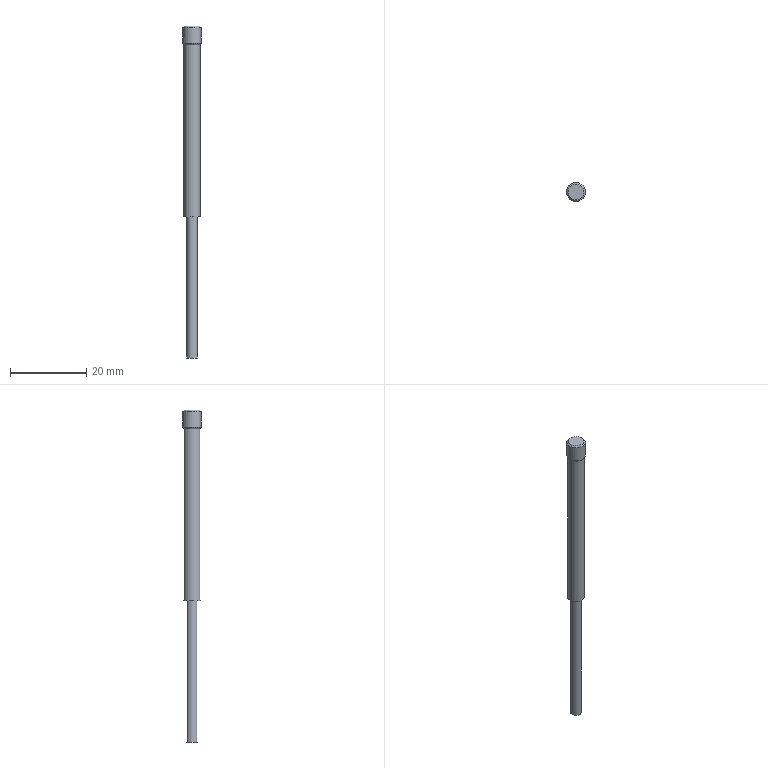Part | NX | features MI_APJAL_0242 2 | 1 solid | 9 faces | box 4.9 x 4.9 x 87 mm | volume 1004 mm3 | cylinder 3 | plane 3 | spline 2 | cone 1 | commonest cylinder face diameters 2.8 x1 4.4 x1 4.9 x1
STEP:
#1=CARTESIAN_POINT('',(146.8,-140.,73.1));
#2=VERTEX_POINT('',#1);
#3=CARTESIAN_POINT('',(151.2,-140.,73.1));
#4=VERTEX_POINT('',#3);
#5=CARTESIAN_POINT('',(149.,-140.,73.1));
#6=DIRECTION('',(0.,0.,1.));
#7=DIRECTION('',(1.,0.,0.));
#8=AXIS2_PLACEMENT_3D('',#5,#6,#7);
#9=CIRCLE('',#8,2.2);
#10=EDGE_CURVE('',#2,#4,#9,.T.);
#11=ORIENTED_EDGE('',*,*,#10,.T.);
#12=CARTESIAN_POINT('',(151.2,-139.998,73.1));
#13=VERTEX_POINT('',#12);
#14=CARTESIAN_POINT('',(149.,-140.,73.1));
#15=DIRECTION('',(0.,0.,1.));
#16=DIRECTION('',(1.,0.,0.));
#17=AXIS2_PLACEMENT_3D('',#14,#15,#16);
#18=CIRCLE('',#17,2.2);
#19=EDGE_CURVE('',#4,#13,#18,.T.);
#20=ORIENTED_EDGE('',*,*,#19,.T.);
#21=CARTESIAN_POINT('',(151.45,-139.998,73.448));
#22=VERTEX_POINT('',#21);
#23=CARTESIAN_POINT('',(151.45,-139.998,73.448));
#24=DIRECTION('',(-0.5832,-0.0004724,-0.8123));
#25=VECTOR('',#24,1000.);
#26=LINE('',#23,#25);
#27=EDGE_CURVE('',#22,#13,#26,.T.);
#28=ORIENTED_EDGE('',*,*,#27,.F.);
#29=CARTESIAN_POINT('',(151.45,-140.,73.448));
#30=VERTEX_POINT('',#29);
#31=CARTESIAN_POINT('',(151.45,-139.998,73.448));
#32=CARTESIAN_POINT('',(151.45,-139.999,73.448));
#33=CARTESIAN_POINT('',(151.45,-139.999,73.448));
#34=CARTESIAN_POINT('',(151.45,-140.,73.448));
#35=B_SPLINE_CURVE_WITH_KNOTS('',3,(#31,#32,#33,#34),.UNSPECIFIED.,.F.,.F.,(4,4),(13.004,13.006),.UNSPECIFIED.);
#36=EDGE_CURVE('',#22,#30,#35,.T.);
#37=ORIENTED_EDGE('',*,*,#36,.T.);
#38=CARTESIAN_POINT('',(148.979,-142.45,73.448));
#39=VERTEX_POINT('',#38);
#40=CARTESIAN_POINT('',(151.45,-140.,73.448));
#41=CARTESIAN_POINT('',(151.45,-140.316,73.448));
#42=CARTESIAN_POINT('',(151.387,-140.638,73.448));
#43=CARTESIAN_POINT('',(151.147,-141.223,73.448));
#44=CARTESIAN_POINT('',(150.966,-141.496,73.448));
#45=CARTESIAN_POINT('',(150.522,-141.946,73.448));
#46=CARTESIAN_POINT('',(150.251,-142.13,73.448));
#47=CARTESIAN_POINT('',(149.669,-142.378,73.448));
#48=CARTESIAN_POINT('',(149.348,-142.446,73.448));
#49=CARTESIAN_POINT('',(149.014,-142.45,73.448));
#50=CARTESIAN_POINT('',(148.996,-142.45,73.448));
#51=CARTESIAN_POINT('',(148.979,-142.45,73.448));
#52=B_SPLINE_CURVE_WITH_KNOTS('',3,(#40,#41,#42,#43,#44,#45,#46,#47,#48,#49,#50,#51),.UNSPECIFIED.,.F.,.F.,(4,2,2,2,2,4),(0.,0.8058,1.612,2.418,3.223,3.269),.UNSPECIFIED.);
#53=EDGE_CURVE('',#30,#39,#52,.T.);
#54=ORIENTED_EDGE('',*,*,#53,.T.);
#55=CARTESIAN_POINT('',(146.55,-140.,73.448));
#56=VERTEX_POINT('',#55);
#57=CARTESIAN_POINT('',(148.979,-142.45,73.448));
#58=CARTESIAN_POINT('',(148.68,-142.447,73.448));
#59=CARTESIAN_POINT('',(148.377,-142.388,73.448));
#60=CARTESIAN_POINT('',(147.806,-142.162,73.448));
#61=CARTESIAN_POINT('',(147.53,-141.985,73.448));
#62=CARTESIAN_POINT('',(147.074,-141.547,73.448));
#63=CARTESIAN_POINT('',(146.886,-141.278,73.448));
#64=CARTESIAN_POINT('',(146.631,-140.7,73.448));
#65=CARTESIAN_POINT('',(146.559,-140.38,73.448));
#66=CARTESIAN_POINT('',(146.55,-140.043,73.448));
#67=CARTESIAN_POINT('',(146.55,-140.021,73.448));
#68=CARTESIAN_POINT('',(146.55,-140.,73.448));
#69=B_SPLINE_CURVE_WITH_KNOTS('',3,(#57,#58,#59,#60,#61,#62,#63,#64,#65,#66,#67,#68),.UNSPECIFIED.,.F.,.F.,(4,2,2,2,2,4),(3.269,4.029,4.835,5.641,6.447,6.501),.UNSPECIFIED.);
#70=EDGE_CURVE('',#39,#56,#69,.T.);
#71=ORIENTED_EDGE('',*,*,#70,.T.);
#72=CARTESIAN_POINT('',(146.8,-140.,73.1));
#73=CARTESIAN_POINT('',(146.717,-140.,73.216));
#74=CARTESIAN_POINT('',(146.634,-140.,73.332));
#75=CARTESIAN_POINT('',(146.55,-140.,73.449));
#76=B_SPLINE_CURVE_WITH_KNOTS('',3,(#72,#73,#74,#75),.UNSPECIFIED.,.F.,.F.,(4,4),(0.,1.),.UNSPECIFIED.);
#77=EDGE_CURVE('',#2,#56,#76,.T.);
#78=ORIENTED_EDGE('',*,*,#77,.F.);
#79=EDGE_LOOP('',(#11,#20,#28,#37,#54,#71,#78));
#80=FACE_BOUND('',#79,.T.);
#81=CARTESIAN_POINT('',(146.8,-140.,73.1));
#82=CARTESIAN_POINT('',(146.717,-140.,73.216));
#83=CARTESIAN_POINT('',(146.634,-140.,73.332));
#84=CARTESIAN_POINT('',(146.55,-140.,73.449));
#85=CARTESIAN_POINT('',(146.8,-140.162,73.1));
#86=CARTESIAN_POINT('',(146.717,-140.168,73.216));
#87=CARTESIAN_POINT('',(146.634,-140.174,73.332));
#88=CARTESIAN_POINT('',(146.55,-140.18,73.449));
#89=CARTESIAN_POINT('',(146.818,-140.324,73.1));
#90=CARTESIAN_POINT('',(146.736,-140.337,73.216));
#91=CARTESIAN_POINT('',(146.653,-140.349,73.332));
#92=CARTESIAN_POINT('',(146.571,-140.361,73.449));
#93=CARTESIAN_POINT('',(146.889,-140.64,73.1));
#94=CARTESIAN_POINT('',(146.809,-140.664,73.216));
#95=CARTESIAN_POINT('',(146.729,-140.688,73.332));
#96=CARTESIAN_POINT('',(146.65,-140.713,73.449));
#97=CARTESIAN_POINT('',(146.943,-140.795,73.1));
#98=CARTESIAN_POINT('',(146.865,-140.825,73.216));
#99=CARTESIAN_POINT('',(146.787,-140.855,73.332));
#100=CARTESIAN_POINT('',(146.709,-140.885,73.449));
#101=CARTESIAN_POINT('',(147.133,-141.197,73.1));
#102=CARTESIAN_POINT('',(147.062,-141.243,73.216));
#103=CARTESIAN_POINT('',(146.992,-141.288,73.332));
#104=CARTESIAN_POINT('',(146.921,-141.333,73.449));
#105=CARTESIAN_POINT('',(147.308,-141.434,73.1));
#106=CARTESIAN_POINT('',(147.244,-141.489,73.216));
#107=CARTESIAN_POINT('',(147.18,-141.543,73.332));
#108=CARTESIAN_POINT('',(147.116,-141.597,73.449));
#109=CARTESIAN_POINT('',(147.728,-141.817,73.1));
#110=CARTESIAN_POINT('',(147.679,-141.885,73.216));
#111=CARTESIAN_POINT('',(147.631,-141.954,73.332));
#112=CARTESIAN_POINT('',(147.583,-142.023,73.448));
#113=CARTESIAN_POINT('',(147.98,-141.969,73.1));
#114=CARTESIAN_POINT('',(147.941,-142.044,73.216));
#115=CARTESIAN_POINT('',(147.902,-142.118,73.332));
#116=CARTESIAN_POINT('',(147.864,-142.193,73.448));
#117=CARTESIAN_POINT('',(148.513,-142.164,73.1));
#118=CARTESIAN_POINT('',(148.494,-142.246,73.216));
#119=CARTESIAN_POINT('',(148.476,-142.328,73.332));
#120=CARTESIAN_POINT('',(148.457,-142.41,73.448));
#121=CARTESIAN_POINT('',(148.804,-142.209,73.1));
#122=CARTESIAN_POINT('',(148.796,-142.293,73.216));
#123=CARTESIAN_POINT('',(148.789,-142.377,73.332));
#124=CARTESIAN_POINT('',(148.781,-142.46,73.448));
#125=CARTESIAN_POINT('',(149.371,-142.187,73.1));
#126=CARTESIAN_POINT('',(149.385,-142.27,73.216));
#127=CARTESIAN_POINT('',(149.399,-142.353,73.332));
#128=CARTESIAN_POINT('',(149.413,-142.435,73.448));
#129=CARTESIAN_POINT('',(149.657,-142.119,73.1));
#130=CARTESIAN_POINT('',(149.682,-142.199,73.216));
#131=CARTESIAN_POINT('',(149.707,-142.279,73.332));
#132=CARTESIAN_POINT('',(149.732,-142.359,73.448));
#133=CARTESIAN_POINT('',(150.173,-141.883,73.1));
#134=CARTESIAN_POINT('',(150.218,-141.954,73.216));
#135=CARTESIAN_POINT('',(150.262,-142.025,73.332));
#136=CARTESIAN_POINT('',(150.307,-142.097,73.448));
#137=CARTESIAN_POINT('',(150.412,-141.711,73.1));
#138=CARTESIAN_POINT('',(150.466,-141.775,73.216));
#139=CARTESIAN_POINT('',(150.519,-141.84,73.332));
#140=CARTESIAN_POINT('',(150.573,-141.905,73.448));
#141=CARTESIAN_POINT('',(150.8,-141.296,73.1));
#142=CARTESIAN_POINT('',(150.868,-141.345,73.216));
#143=CARTESIAN_POINT('',(150.937,-141.395,73.332));
#144=CARTESIAN_POINT('',(151.005,-141.444,73.448));
#145=CARTESIAN_POINT('',(150.956,-141.046,73.1));
#146=CARTESIAN_POINT('',(151.03,-141.086,73.216));
#147=CARTESIAN_POINT('',(151.104,-141.126,73.332));
#148=CARTESIAN_POINT('',(151.178,-141.165,73.448));
#149=CARTESIAN_POINT('',(151.158,-140.516,73.1));
#150=CARTESIAN_POINT('',(151.239,-140.535,73.216));
#151=CARTESIAN_POINT('',(151.321,-140.555,73.332));
#152=CARTESIAN_POINT('',(151.403,-140.575,73.448));
#153=CARTESIAN_POINT('',(151.207,-140.226,73.1));
#154=CARTESIAN_POINT('',(151.291,-140.234,73.216));
#155=CARTESIAN_POINT('',(151.374,-140.243,73.332));
#156=CARTESIAN_POINT('',(151.458,-140.251,73.448));
#157=CARTESIAN_POINT('',(151.192,-139.658,73.1));
#158=CARTESIAN_POINT('',(151.275,-139.645,73.216));
#159=CARTESIAN_POINT('',(151.358,-139.632,73.332));
#160=CARTESIAN_POINT('',(151.441,-139.619,73.448));
#161=CARTESIAN_POINT('',(151.128,-139.371,73.1));
#162=CARTESIAN_POINT('',(151.208,-139.347,73.216));
#163=CARTESIAN_POINT('',(151.289,-139.323,73.332));
#164=CARTESIAN_POINT('',(151.369,-139.299,73.448));
#165=CARTESIAN_POINT('',(150.898,-138.852,73.1));
#166=CARTESIAN_POINT('',(150.97,-138.808,73.216));
#167=CARTESIAN_POINT('',(151.042,-138.765,73.332));
#168=CARTESIAN_POINT('',(151.114,-138.721,73.448));
#169=CARTESIAN_POINT('',(150.73,-138.61,73.1));
#170=CARTESIAN_POINT('',(150.795,-138.558,73.216));
#171=CARTESIAN_POINT('',(150.861,-138.505,73.332));
#172=CARTESIAN_POINT('',(150.926,-138.452,73.448));
#173=CARTESIAN_POINT('',(150.32,-138.217,73.1));
#174=CARTESIAN_POINT('',(150.37,-138.15,73.216));
#175=CARTESIAN_POINT('',(150.42,-138.082,73.332));
#176=CARTESIAN_POINT('',(150.47,-138.014,73.448));
#177=CARTESIAN_POINT('',(150.073,-138.058,73.1));
#178=CARTESIAN_POINT('',(150.113,-137.984,73.216));
#179=CARTESIAN_POINT('',(150.154,-137.911,73.332));
#180=CARTESIAN_POINT('',(150.194,-137.837,73.448));
#181=CARTESIAN_POINT('',(149.545,-137.849,73.1));
#182=CARTESIAN_POINT('',(149.565,-137.768,73.216));
#183=CARTESIAN_POINT('',(149.586,-137.687,73.332));
#184=CARTESIAN_POINT('',(149.607,-137.605,73.448));
#185=CARTESIAN_POINT('',(149.255,-137.796,73.1));
#186=CARTESIAN_POINT('',(149.265,-137.713,73.216));
#187=CARTESIAN_POINT('',(149.274,-137.629,73.332));
#188=CARTESIAN_POINT('',(149.284,-137.546,73.448));
#189=CARTESIAN_POINT('',(148.688,-137.804,73.1));
#190=CARTESIAN_POINT('',(148.676,-137.721,73.216));
#191=CARTESIAN_POINT('',(148.664,-137.637,73.332));
#192=CARTESIAN_POINT('',(148.652,-137.554,73.448));
#193=CARTESIAN_POINT('',(148.399,-137.865,73.1));
#194=CARTESIAN_POINT('',(148.377,-137.784,73.216));
#195=CARTESIAN_POINT('',(148.354,-137.703,73.332));
#196=CARTESIAN_POINT('',(148.331,-137.622,73.448));
#197=CARTESIAN_POINT('',(147.877,-138.087,73.1));
#198=CARTESIAN_POINT('',(147.835,-138.015,73.216));
#199=CARTESIAN_POINT('',(147.792,-137.942,73.332));
#200=CARTESIAN_POINT('',(147.75,-137.87,73.448));
#201=CARTESIAN_POINT('',(147.634,-138.253,73.1));
#202=CARTESIAN_POINT('',(147.582,-138.186,73.216));
#203=CARTESIAN_POINT('',(147.53,-138.12,73.332));
#204=CARTESIAN_POINT('',(147.478,-138.054,73.448));
#205=CARTESIAN_POINT('',(147.235,-138.657,73.1));
#206=CARTESIAN_POINT('',(147.168,-138.606,73.216));
#207=CARTESIAN_POINT('',(147.101,-138.555,73.332));
#208=CARTESIAN_POINT('',(147.035,-138.504,73.448));
#209=CARTESIAN_POINT('',(147.073,-138.902,73.1));
#210=CARTESIAN_POINT('',(147.,-138.861,73.216));
#211=CARTESIAN_POINT('',(146.927,-138.819,73.332));
#212=CARTESIAN_POINT('',(146.854,-138.778,73.448));
#213=CARTESIAN_POINT('',(146.857,-139.427,73.1));
#214=CARTESIAN_POINT('',(146.776,-139.406,73.216));
#215=CARTESIAN_POINT('',(146.695,-139.384,73.332));
#216=CARTESIAN_POINT('',(146.614,-139.362,73.448));
#217=CARTESIAN_POINT('',(146.8,-139.716,73.1));
#218=CARTESIAN_POINT('',(146.717,-139.706,73.216));
#219=CARTESIAN_POINT('',(146.634,-139.695,73.332));
#220=CARTESIAN_POINT('',(146.55,-139.684,73.448));
#221=CARTESIAN_POINT('',(146.8,-140.,73.1));
#222=CARTESIAN_POINT('',(146.717,-140.,73.216));
#223=CARTESIAN_POINT('',(146.634,-140.,73.332));
#224=CARTESIAN_POINT('',(146.55,-140.,73.449));
#225=B_SPLINE_SURFACE_WITH_KNOTS('',3,3,((#81,#82,#83,#84),(#85,#86,#87,#88),(#89,#90,#91,#92),(#93,#94,#95,#96),(#97,#98,#99,#100),(#101,#102,#103,#104),(#105,#106,#107,#108),(#109,#110,#111,#112),(#113,#114,#115,#116),(#117,#118,#119,#120),(#121,#122,#123,#124),(#125,#126,#127,#128),(#129,#130,#131,#132),(#133,#134,#135,#136),(#137,#138,#139,#140),(#141,#142,#143,#144),(#145,#146,#147,#148),(#149,#150,#151,#152),(#153,#154,#155,#156),(#157,#158,#159,#160),(#161,#162,#163,#164),(#165,#166,#167,#168),(#169,#170,#171,#172),(#173,#174,#175,#176),(#177,#178,#179,#180),(#181,#182,#183,#184),(#185,#186,#187,#188),(#189,#190,#191,#192),(#193,#194,#195,#196),(#197,#198,#199,#200),(#201,#202,#203,#204),(#205,#206,#207,#208),(#209,#210,#211,#212),(#213,#214,#215,#216),(#217,#218,#219,#220),(#221,#222,#223,#224)),.RULED_SURF.,.T.,.F.,.F.,(4,2,2,2,2,2,2,2,2,2,2,2,2,2,2,2,2,4),(4,4),(-13.006,-12.547,-12.088,-11.282,-10.476,-9.67,-8.864,-8.058,-7.253,-6.447,-5.641,-4.835,-4.029,-3.223,-2.418,-1.612,-0.8058,0.),(0.,1.),.UNSPECIFIED.);
#226=ADVANCED_FACE('',(#80),#225,.T.);
#227=CARTESIAN_POINT('',(151.45,-140.014,77.632));
#228=VERTEX_POINT('',#227);
#229=CARTESIAN_POINT('',(146.55,-140.,77.632));
#230=VERTEX_POINT('',#229);
#231=CARTESIAN_POINT('',(149.,-140.,77.632));
#232=DIRECTION('',(0.,0.,1.));
#233=DIRECTION('',(-1.,0.,0.));
#234=AXIS2_PLACEMENT_3D('',#231,#232,#233);
#235=CIRCLE('',#234,2.45);
#236=EDGE_CURVE('',#228,#230,#235,.T.);
#237=ORIENTED_EDGE('',*,*,#236,.F.);
#238=CARTESIAN_POINT('',(148.979,-142.45,77.632));
#239=VERTEX_POINT('',#238);
#240=CARTESIAN_POINT('',(149.,-140.,77.632));
#241=DIRECTION('',(0.,0.,1.));
#242=DIRECTION('',(-1.,0.,0.));
#243=AXIS2_PLACEMENT_3D('',#240,#241,#242);
#244=CIRCLE('',#243,2.45);
#245=EDGE_CURVE('',#239,#228,#244,.T.);
#246=ORIENTED_EDGE('',*,*,#245,.F.);
#247=CARTESIAN_POINT('',(148.979,-142.45,77.632));
#248=CARTESIAN_POINT('',(148.979,-142.45,73.448));
#249=B_SPLINE_CURVE_WITH_KNOTS('',1,(#247,#248),.UNSPECIFIED.,.F.,.F.,(2,2),(0.08333,0.9167),.UNSPECIFIED.);
#250=EDGE_CURVE('',#239,#39,#249,.T.);
#251=ORIENTED_EDGE('',*,*,#250,.T.);
#252=ORIENTED_EDGE('',*,*,#53,.F.);
#253=ORIENTED_EDGE('',*,*,#36,.F.);
#254=CARTESIAN_POINT('',(146.55,-140.,73.448));
#255=CARTESIAN_POINT('',(146.55,-139.705,73.448));
#256=CARTESIAN_POINT('',(146.605,-139.405,73.448));
#257=CARTESIAN_POINT('',(146.822,-138.834,73.448));
#258=CARTESIAN_POINT('',(146.996,-138.556,73.448));
#259=CARTESIAN_POINT('',(147.428,-138.095,73.448));
#260=CARTESIAN_POINT('',(147.694,-137.903,73.448));
#261=CARTESIAN_POINT('',(148.269,-137.64,73.448));
#262=CARTESIAN_POINT('',(148.588,-137.564,73.448));
#263=CARTESIAN_POINT('',(149.219,-137.539,73.448));
#264=CARTESIAN_POINT('',(149.543,-137.59,73.448));
#265=CARTESIAN_POINT('',(150.137,-137.807,73.448));
#266=CARTESIAN_POINT('',(150.418,-137.977,73.448));
#267=CARTESIAN_POINT('',(150.885,-138.403,73.448));
#268=CARTESIAN_POINT('',(151.079,-138.667,73.448));
#269=CARTESIAN_POINT('',(151.292,-139.115,73.448));
#270=CARTESIAN_POINT('',(151.351,-139.287,73.448));
#271=CARTESIAN_POINT('',(151.43,-139.638,73.448));
#272=CARTESIAN_POINT('',(151.45,-139.819,73.448));
#273=CARTESIAN_POINT('',(151.45,-139.998,73.448));
#274=B_SPLINE_CURVE_WITH_KNOTS('',3,(#254,#255,#256,#257,#258,#259,#260,#261,#262,#263,#264,#265,#266,#267,#268,#269,#270,#271,#272,#273),.UNSPECIFIED.,.F.,.F.,(4,2,2,2,2,2,2,2,2,4),(6.501,7.253,8.058,8.864,9.67,10.476,11.282,12.088,12.547,13.004),.UNSPECIFIED.);
#275=EDGE_CURVE('',#56,#22,#274,.T.);
#276=ORIENTED_EDGE('',*,*,#275,.F.);
#277=ORIENTED_EDGE('',*,*,#70,.F.);
#278=ORIENTED_EDGE('',*,*,#250,.F.);
#279=CARTESIAN_POINT('',(149.,-140.,77.632));
#280=DIRECTION('',(0.,0.,1.));
#281=DIRECTION('',(-1.,0.,0.));
#282=AXIS2_PLACEMENT_3D('',#279,#280,#281);
#283=CIRCLE('',#282,2.45);
#284=EDGE_CURVE('',#230,#239,#283,.T.);
#285=ORIENTED_EDGE('',*,*,#284,.F.);
#286=EDGE_LOOP('',(#237,#246,#251,#252,#253,#276,#277,#278,#285));
#287=FACE_BOUND('',#286,.T.);
#288=CARTESIAN_POINT('',(149.,-140.,75.55));
#289=DIRECTION('',(0.,0.,-1.));
#290=DIRECTION('',(-0.008727,-1.,0.));
#291=AXIS2_PLACEMENT_3D('',#288,#289,#290);
#292=CYLINDRICAL_SURFACE('',#291,2.45);
#293=ADVANCED_FACE('',(#287),#292,.T.);
#294=CARTESIAN_POINT('',(146.917,-140.,78.));
#295=VERTEX_POINT('',#294);
#296=CARTESIAN_POINT('',(151.082,-140.012,78.));
#297=VERTEX_POINT('',#296);
#298=CARTESIAN_POINT('',(149.,-140.,78.));
#299=DIRECTION('',(0.,0.,-1.));
#300=DIRECTION('',(-1.,0.,0.));
#301=AXIS2_PLACEMENT_3D('',#298,#299,#300);
#302=CIRCLE('',#301,2.083);
#303=EDGE_CURVE('',#295,#297,#302,.T.);
#304=ORIENTED_EDGE('',*,*,#303,.T.);
#305=CARTESIAN_POINT('',(151.082,-140.012,78.));
#306=CARTESIAN_POINT('',(151.45,-140.014,77.633));
#307=B_SPLINE_CURVE_WITH_KNOTS('',1,(#305,#306),.UNSPECIFIED.,.F.,.F.,(2,2),(0.601,0.7071),.UNSPECIFIED.);
#308=EDGE_CURVE('',#297,#228,#307,.T.);
#309=ORIENTED_EDGE('',*,*,#308,.T.);
#310=ORIENTED_EDGE('',*,*,#236,.T.);
#311=ORIENTED_EDGE('',*,*,#284,.T.);
#312=ORIENTED_EDGE('',*,*,#245,.T.);
#313=ORIENTED_EDGE('',*,*,#308,.F.);
#314=CARTESIAN_POINT('',(149.,-140.,78.));
#315=DIRECTION('',(0.,0.,-1.));
#316=DIRECTION('',(-1.,0.,0.));
#317=AXIS2_PLACEMENT_3D('',#314,#315,#316);
#318=CIRCLE('',#317,2.083);
#319=EDGE_CURVE('',#297,#295,#318,.T.);
#320=ORIENTED_EDGE('',*,*,#319,.T.);
#321=EDGE_LOOP('',(#304,#309,#310,#311,#312,#313,#320));
#322=FACE_BOUND('',#321,.T.);
#323=CARTESIAN_POINT('',(149.,-140.,76.618));
#324=DIRECTION('',(0.,0.,-1.));
#325=DIRECTION('',(1.,-0.005818,0.));
#326=AXIS2_PLACEMENT_3D('',#323,#324,#325);
#327=CONICAL_SURFACE('',#326,3.465,0.7854);
#328=ADVANCED_FACE('',(#322),#327,.T.);
#329=ORIENTED_EDGE('',*,*,#319,.F.);
#330=ORIENTED_EDGE('',*,*,#303,.F.);
#331=EDGE_LOOP('',(#329,#330));
#332=FACE_BOUND('',#331,.T.);
#333=CARTESIAN_POINT('',(146.293,-144.328,78.));
#334=DIRECTION('',(0.,0.,1.));
#335=DIRECTION('',(1.,0.,0.));
#336=AXIS2_PLACEMENT_3D('',#333,#334,#335);
#337=PLANE('',#336);
#338=ADVANCED_FACE('',(#332),#337,.T.);
#339=CARTESIAN_POINT('',(147.6,-140.,28.));
#340=VERTEX_POINT('',#339);
#341=CARTESIAN_POINT('',(149.,-140.,28.));
#342=DIRECTION('',(0.,0.,1.));
#343=DIRECTION('',(-1.,0.,0.));
#344=AXIS2_PLACEMENT_3D('',#341,#342,#343);
#345=CIRCLE('',#344,1.4);
#346=EDGE_CURVE('',#340,#340,#345,.T.);
#347=ORIENTED_EDGE('',*,*,#346,.F.);
#348=CARTESIAN_POINT('',(147.6,-140.,-9.));
#349=VERTEX_POINT('',#348);
#350=CARTESIAN_POINT('',(147.6,-140.,28.));
#351=CARTESIAN_POINT('',(147.6,-140.,-9.));
#352=B_SPLINE_CURVE_WITH_KNOTS('',1,(#350,#351),.UNSPECIFIED.,.F.,.F.,(2,2),(0.08333,0.9167),.UNSPECIFIED.);
#353=EDGE_CURVE('',#340,#349,#352,.T.);
#354=ORIENTED_EDGE('',*,*,#353,.T.);
#355=CARTESIAN_POINT('',(149.,-140.,-9.));
#356=DIRECTION('',(0.,0.,-1.));
#357=DIRECTION('',(-1.,0.,0.));
#358=AXIS2_PLACEMENT_3D('',#355,#356,#357);
#359=CIRCLE('',#358,1.4);
#360=EDGE_CURVE('',#349,#349,#359,.T.);
#361=ORIENTED_EDGE('',*,*,#360,.F.);
#362=ORIENTED_EDGE('',*,*,#353,.F.);
#363=EDGE_LOOP('',(#347,#354,#361,#362));
#364=FACE_BOUND('',#363,.T.);
#365=CARTESIAN_POINT('',(149.,-140.,9.5));
#366=DIRECTION('',(0.,0.,-1.));
#367=DIRECTION('',(-1.,0.,0.));
#368=AXIS2_PLACEMENT_3D('',#365,#366,#367);
#369=CYLINDRICAL_SURFACE('',#368,1.4);
#370=ADVANCED_FACE('',(#364),#369,.T.);
#371=ORIENTED_EDGE('',*,*,#360,.T.);
#372=EDGE_LOOP('',(#371));
#373=FACE_BOUND('',#372,.T.);
#374=CARTESIAN_POINT('',(152.22,-142.91,-9.));
#375=DIRECTION('',(0.,0.,-1.));
#376=DIRECTION('',(-1.,0.,0.));
#377=AXIS2_PLACEMENT_3D('',#374,#375,#376);
#378=PLANE('',#377);
#379=ADVANCED_FACE('',(#373),#378,.T.);
#380=ORIENTED_EDGE('',*,*,#10,.F.);
#381=CARTESIAN_POINT('',(146.8,-140.,28.));
#382=VERTEX_POINT('',#381);
#383=CARTESIAN_POINT('',(146.8,-140.,73.1));
#384=CARTESIAN_POINT('',(146.8,-140.,28.));
#385=B_SPLINE_CURVE_WITH_KNOTS('',1,(#383,#384),.UNSPECIFIED.,.F.,.F.,(2,2),(0.08333,0.9167),.UNSPECIFIED.);
#386=EDGE_CURVE('',#2,#382,#385,.T.);
#387=ORIENTED_EDGE('',*,*,#386,.T.);
#388=CARTESIAN_POINT('',(149.,-140.,28.));
#389=DIRECTION('',(0.,0.,-1.));
#390=DIRECTION('',(-1.,0.,0.));
#391=AXIS2_PLACEMENT_3D('',#388,#389,#390);
#392=CIRCLE('',#391,2.2);
#393=EDGE_CURVE('',#382,#382,#392,.T.);
#394=ORIENTED_EDGE('',*,*,#393,.F.);
#395=ORIENTED_EDGE('',*,*,#386,.F.);
#396=CARTESIAN_POINT('',(149.,-140.,73.1));
#397=DIRECTION('',(0.,0.,1.));
#398=DIRECTION('',(1.,0.,0.));
#399=AXIS2_PLACEMENT_3D('',#396,#397,#398);
#400=CIRCLE('',#399,2.2);
#401=EDGE_CURVE('',#13,#2,#400,.T.);
#402=ORIENTED_EDGE('',*,*,#401,.F.);
#403=ORIENTED_EDGE('',*,*,#19,.F.);
#404=EDGE_LOOP('',(#380,#387,#394,#395,#402,#403));
#405=FACE_BOUND('',#404,.T.);
#406=CARTESIAN_POINT('',(149.,-140.,50.55));
#407=DIRECTION('',(0.,0.,-1.));
#408=DIRECTION('',(-1.,0.,0.));
#409=AXIS2_PLACEMENT_3D('',#406,#407,#408);
#410=CYLINDRICAL_SURFACE('',#409,2.2);
#411=ADVANCED_FACE('',(#405),#410,.T.);
#412=ORIENTED_EDGE('',*,*,#393,.T.);
#413=EDGE_LOOP('',(#412));
#414=FACE_BOUND('',#413,.T.);
#415=ORIENTED_EDGE('',*,*,#346,.T.);
#416=EDGE_LOOP('',(#415));
#417=FACE_BOUND('',#416,.T.);
#418=CARTESIAN_POINT('',(154.06,-144.573,28.));
#419=DIRECTION('',(0.,0.,-1.));
#420=DIRECTION('',(-1.,0.,0.));
#421=AXIS2_PLACEMENT_3D('',#418,#419,#420);
#422=PLANE('',#421);
#423=ADVANCED_FACE('',(#414,#417),#422,.T.);
#424=ORIENTED_EDGE('',*,*,#275,.T.);
#425=ORIENTED_EDGE('',*,*,#27,.T.);
#426=ORIENTED_EDGE('',*,*,#401,.T.);
#427=ORIENTED_EDGE('',*,*,#77,.T.);
#428=EDGE_LOOP('',(#424,#425,#426,#427));
#429=FACE_BOUND('',#428,.T.);
#430=CARTESIAN_POINT('',(146.8,-140.,73.1));
#431=CARTESIAN_POINT('',(146.717,-140.,73.216));
#432=CARTESIAN_POINT('',(146.634,-140.,73.332));
#433=CARTESIAN_POINT('',(146.55,-140.,73.449));
#434=CARTESIAN_POINT('',(146.8,-140.162,73.1));
#435=CARTESIAN_POINT('',(146.717,-140.168,73.216));
#436=CARTESIAN_POINT('',(146.634,-140.174,73.332));
#437=CARTESIAN_POINT('',(146.55,-140.18,73.449));
#438=CARTESIAN_POINT('',(146.818,-140.324,73.1));
#439=CARTESIAN_POINT('',(146.736,-140.337,73.216));
#440=CARTESIAN_POINT('',(146.653,-140.349,73.332));
#441=CARTESIAN_POINT('',(146.571,-140.361,73.449));
#442=CARTESIAN_POINT('',(146.889,-140.64,73.1));
#443=CARTESIAN_POINT('',(146.809,-140.664,73.216));
#444=CARTESIAN_POINT('',(146.729,-140.688,73.332));
#445=CARTESIAN_POINT('',(146.65,-140.713,73.449));
#446=CARTESIAN_POINT('',(146.943,-140.795,73.1));
#447=CARTESIAN_POINT('',(146.865,-140.825,73.216));
#448=CARTESIAN_POINT('',(146.787,-140.855,73.332));
#449=CARTESIAN_POINT('',(146.709,-140.885,73.449));
#450=CARTESIAN_POINT('',(147.133,-141.197,73.1));
#451=CARTESIAN_POINT('',(147.062,-141.243,73.216));
#452=CARTESIAN_POINT('',(146.992,-141.288,73.332));
#453=CARTESIAN_POINT('',(146.921,-141.333,73.449));
#454=CARTESIAN_POINT('',(147.308,-141.434,73.1));
#455=CARTESIAN_POINT('',(147.244,-141.489,73.216));
#456=CARTESIAN_POINT('',(147.18,-141.543,73.332));
#457=CARTESIAN_POINT('',(147.116,-141.597,73.449));
#458=CARTESIAN_POINT('',(147.728,-141.817,73.1));
#459=CARTESIAN_POINT('',(147.679,-141.885,73.216));
#460=CARTESIAN_POINT('',(147.631,-141.954,73.332));
#461=CARTESIAN_POINT('',(147.583,-142.023,73.448));
#462=CARTESIAN_POINT('',(147.98,-141.969,73.1));
#463=CARTESIAN_POINT('',(147.941,-142.044,73.216));
#464=CARTESIAN_POINT('',(147.902,-142.118,73.332));
#465=CARTESIAN_POINT('',(147.864,-142.193,73.448));
#466=CARTESIAN_POINT('',(148.513,-142.164,73.1));
#467=CARTESIAN_POINT('',(148.494,-142.246,73.216));
#468=CARTESIAN_POINT('',(148.476,-142.328,73.332));
#469=CARTESIAN_POINT('',(148.457,-142.41,73.448));
#470=CARTESIAN_POINT('',(148.804,-142.209,73.1));
#471=CARTESIAN_POINT('',(148.796,-142.293,73.216));
#472=CARTESIAN_POINT('',(148.789,-142.377,73.332));
#473=CARTESIAN_POINT('',(148.781,-142.46,73.448));
#474=CARTESIAN_POINT('',(149.371,-142.187,73.1));
#475=CARTESIAN_POINT('',(149.385,-142.27,73.216));
#476=CARTESIAN_POINT('',(149.399,-142.353,73.332));
#477=CARTESIAN_POINT('',(149.413,-142.435,73.448));
#478=CARTESIAN_POINT('',(149.657,-142.119,73.1));
#479=CARTESIAN_POINT('',(149.682,-142.199,73.216));
#480=CARTESIAN_POINT('',(149.707,-142.279,73.332));
#481=CARTESIAN_POINT('',(149.732,-142.359,73.448));
#482=CARTESIAN_POINT('',(150.173,-141.883,73.1));
#483=CARTESIAN_POINT('',(150.218,-141.954,73.216));
#484=CARTESIAN_POINT('',(150.262,-142.025,73.332));
#485=CARTESIAN_POINT('',(150.307,-142.097,73.448));
#486=CARTESIAN_POINT('',(150.412,-141.711,73.1));
#487=CARTESIAN_POINT('',(150.466,-141.775,73.216));
#488=CARTESIAN_POINT('',(150.519,-141.84,73.332));
#489=CARTESIAN_POINT('',(150.573,-141.905,73.448));
#490=CARTESIAN_POINT('',(150.8,-141.296,73.1));
#491=CARTESIAN_POINT('',(150.868,-141.345,73.216));
#492=CARTESIAN_POINT('',(150.937,-141.395,73.332));
#493=CARTESIAN_POINT('',(151.005,-141.444,73.448));
#494=CARTESIAN_POINT('',(150.956,-141.046,73.1));
#495=CARTESIAN_POINT('',(151.03,-141.086,73.216));
#496=CARTESIAN_POINT('',(151.104,-141.126,73.332));
#497=CARTESIAN_POINT('',(151.178,-141.165,73.448));
#498=CARTESIAN_POINT('',(151.158,-140.516,73.1));
#499=CARTESIAN_POINT('',(151.239,-140.535,73.216));
#500=CARTESIAN_POINT('',(151.321,-140.555,73.332));
#501=CARTESIAN_POINT('',(151.403,-140.575,73.448));
#502=CARTESIAN_POINT('',(151.207,-140.226,73.1));
#503=CARTESIAN_POINT('',(151.291,-140.234,73.216));
#504=CARTESIAN_POINT('',(151.374,-140.243,73.332));
#505=CARTESIAN_POINT('',(151.458,-140.251,73.448));
#506=CARTESIAN_POINT('',(151.192,-139.658,73.1));
#507=CARTESIAN_POINT('',(151.275,-139.645,73.216));
#508=CARTESIAN_POINT('',(151.358,-139.632,73.332));
#509=CARTESIAN_POINT('',(151.441,-139.619,73.448));
#510=CARTESIAN_POINT('',(151.128,-139.371,73.1));
#511=CARTESIAN_POINT('',(151.208,-139.347,73.216));
#512=CARTESIAN_POINT('',(151.289,-139.323,73.332));
#513=CARTESIAN_POINT('',(151.369,-139.299,73.448));
#514=CARTESIAN_POINT('',(150.898,-138.852,73.1));
#515=CARTESIAN_POINT('',(150.97,-138.808,73.216));
#516=CARTESIAN_POINT('',(151.042,-138.765,73.332));
#517=CARTESIAN_POINT('',(151.114,-138.721,73.448));
#518=CARTESIAN_POINT('',(150.73,-138.61,73.1));
#519=CARTESIAN_POINT('',(150.795,-138.558,73.216));
#520=CARTESIAN_POINT('',(150.861,-138.505,73.332));
#521=CARTESIAN_POINT('',(150.926,-138.452,73.448));
#522=CARTESIAN_POINT('',(150.32,-138.217,73.1));
#523=CARTESIAN_POINT('',(150.37,-138.15,73.216));
#524=CARTESIAN_POINT('',(150.42,-138.082,73.332));
#525=CARTESIAN_POINT('',(150.47,-138.014,73.448));
#526=CARTESIAN_POINT('',(150.073,-138.058,73.1));
#527=CARTESIAN_POINT('',(150.113,-137.984,73.216));
#528=CARTESIAN_POINT('',(150.154,-137.911,73.332));
#529=CARTESIAN_POINT('',(150.194,-137.837,73.448));
#530=CARTESIAN_POINT('',(149.545,-137.849,73.1));
#531=CARTESIAN_POINT('',(149.565,-137.768,73.216));
#532=CARTESIAN_POINT('',(149.586,-137.687,73.332));
#533=CARTESIAN_POINT('',(149.607,-137.605,73.448));
#534=CARTESIAN_POINT('',(149.255,-137.796,73.1));
#535=CARTESIAN_POINT('',(149.265,-137.713,73.216));
#536=CARTESIAN_POINT('',(149.274,-137.629,73.332));
#537=CARTESIAN_POINT('',(149.284,-137.546,73.448));
#538=CARTESIAN_POINT('',(148.688,-137.804,73.1));
#539=CARTESIAN_POINT('',(148.676,-137.721,73.216));
#540=CARTESIAN_POINT('',(148.664,-137.637,73.332));
#541=CARTESIAN_POINT('',(148.652,-137.554,73.448));
#542=CARTESIAN_POINT('',(148.399,-137.865,73.1));
#543=CARTESIAN_POINT('',(148.377,-137.784,73.216));
#544=CARTESIAN_POINT('',(148.354,-137.703,73.332));
#545=CARTESIAN_POINT('',(148.331,-137.622,73.448));
#546=CARTESIAN_POINT('',(147.877,-138.087,73.1));
#547=CARTESIAN_POINT('',(147.835,-138.015,73.216));
#548=CARTESIAN_POINT('',(147.792,-137.942,73.332));
#549=CARTESIAN_POINT('',(147.75,-137.87,73.448));
#550=CARTESIAN_POINT('',(147.634,-138.253,73.1));
#551=CARTESIAN_POINT('',(147.582,-138.186,73.216));
#552=CARTESIAN_POINT('',(147.53,-138.12,73.332));
#553=CARTESIAN_POINT('',(147.478,-138.054,73.448));
#554=CARTESIAN_POINT('',(147.235,-138.657,73.1));
#555=CARTESIAN_POINT('',(147.168,-138.606,73.216));
#556=CARTESIAN_POINT('',(147.101,-138.555,73.332));
#557=CARTESIAN_POINT('',(147.035,-138.504,73.448));
#558=CARTESIAN_POINT('',(147.073,-138.902,73.1));
#559=CARTESIAN_POINT('',(147.,-138.861,73.216));
#560=CARTESIAN_POINT('',(146.927,-138.819,73.332));
#561=CARTESIAN_POINT('',(146.854,-138.778,73.448));
#562=CARTESIAN_POINT('',(146.857,-139.427,73.1));
#563=CARTESIAN_POINT('',(146.776,-139.406,73.216));
#564=CARTESIAN_POINT('',(146.695,-139.384,73.332));
#565=CARTESIAN_POINT('',(146.614,-139.362,73.448));
#566=CARTESIAN_POINT('',(146.8,-139.716,73.1));
#567=CARTESIAN_POINT('',(146.717,-139.706,73.216));
#568=CARTESIAN_POINT('',(146.634,-139.695,73.332));
#569=CARTESIAN_POINT('',(146.55,-139.684,73.448));
#570=CARTESIAN_POINT('',(146.8,-140.,73.1));
#571=CARTESIAN_POINT('',(146.717,-140.,73.216));
#572=CARTESIAN_POINT('',(146.634,-140.,73.332));
#573=CARTESIAN_POINT('',(146.55,-140.,73.449));
#574=B_SPLINE_SURFACE_WITH_KNOTS('',3,3,((#430,#431,#432,#433),(#434,#435,#436,#437),(#438,#439,#440,#441),(#442,#443,#444,#445),(#446,#447,#448,#449),(#450,#451,#452,#453),(#454,#455,#456,#457),(#458,#459,#460,#461),(#462,#463,#464,#465),(#466,#467,#468,#469),(#470,#471,#472,#473),(#474,#475,#476,#477),(#478,#479,#480,#481),(#482,#483,#484,#485),(#486,#487,#488,#489),(#490,#491,#492,#493),(#494,#495,#496,#497),(#498,#499,#500,#501),(#502,#503,#504,#505),(#506,#507,#508,#509),(#510,#511,#512,#513),(#514,#515,#516,#517),(#518,#519,#520,#521),(#522,#523,#524,#525),(#526,#527,#528,#529),(#530,#531,#532,#533),(#534,#535,#536,#537),(#538,#539,#540,#541),(#542,#543,#544,#545),(#546,#547,#548,#549),(#550,#551,#552,#553),(#554,#555,#556,#557),(#558,#559,#560,#561),(#562,#563,#564,#565),(#566,#567,#568,#569),(#570,#571,#572,#573)),.RULED_SURF.,.T.,.F.,.F.,(4,2,2,2,2,2,2,2,2,2,2,2,2,2,2,2,2,4),(4,4),(-13.006,-12.547,-12.088,-11.282,-10.476,-9.67,-8.864,-8.058,-7.253,-6.447,-5.641,-4.835,-4.029,-3.223,-2.418,-1.612,-0.8058,0.),(0.,1.),.UNSPECIFIED.);
#575=ADVANCED_FACE('',(#429),#574,.T.);
#576=CLOSED_SHELL('',(#226,#293,#328,#338,#370,#379,#411,#423,#575));
#577=MANIFOLD_SOLID_BREP('',#576);
#578=(LENGTH_UNIT()NAMED_UNIT(*)SI_UNIT(.MILLI.,.METRE.));
#579=UNCERTAINTY_MEASURE_WITH_UNIT(LENGTH_MEASURE(0.00001),#578,'','');
#580=(NAMED_UNIT(*)PLANE_ANGLE_UNIT()SI_UNIT($,.RADIAN.));
#581=(NAMED_UNIT(*)SI_UNIT($,.STERADIAN.)SOLID_ANGLE_UNIT());
#582=(GEOMETRIC_REPRESENTATION_CONTEXT(3)GLOBAL_UNCERTAINTY_ASSIGNED_CONTEXT((#579))GLOBAL_UNIT_ASSIGNED_CONTEXT((#578,#580,#581))REPRESENTATION_CONTEXT('',''));
#583=ADVANCED_BREP_SHAPE_REPRESENTATION('',(#577),#582);